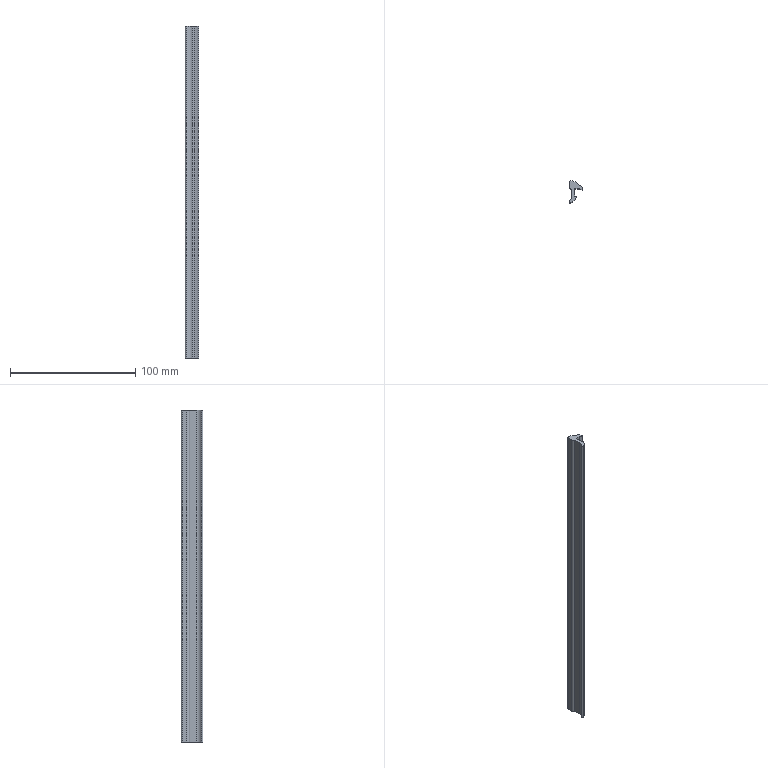Part | SolidWorks | features BaseBody 1, MoveFace 1 | 1 solid | 20 faces | box 10.8 x 17.5 x 265 mm | volume 20882 mm3 | cylinder 11 | plane 9 | commonest cylinder face diameters 1.6 x2 14 x2 0.4 x1 0.6 x1 0.8 x1 2.6 x1
STEP:
#1=CARTESIAN_POINT('',(-3.236,-11.055,165.));
#2=VERTEX_POINT('',#1);
#3=CARTESIAN_POINT('',(-4.3,-10.3,165.));
#4=VERTEX_POINT('',#3);
#5=CARTESIAN_POINT('',(-3.5,-10.3,165.));
#6=DIRECTION('',(0.,0.,-1.));
#7=DIRECTION('',(1.,0.,0.));
#8=AXIS2_PLACEMENT_3D('',#5,#6,#7);
#9=CIRCLE('',#8,0.8);
#10=EDGE_CURVE('',#2,#4,#9,.T.);
#11=ORIENTED_EDGE('',*,*,#10,.T.);
#12=CARTESIAN_POINT('',(-4.3,-10.3,-100.));
#13=VERTEX_POINT('',#12);
#14=CARTESIAN_POINT('',(-4.3,-10.3,-100.));
#15=DIRECTION('',(0.,0.,-1.));
#16=VECTOR('',#15,1000.);
#17=LINE('',#14,#16);
#18=EDGE_CURVE('',#4,#13,#17,.T.);
#19=ORIENTED_EDGE('',*,*,#18,.T.);
#20=CARTESIAN_POINT('',(-3.236,-11.055,-100.));
#21=VERTEX_POINT('',#20);
#22=CARTESIAN_POINT('',(-3.5,-10.3,-100.));
#23=DIRECTION('',(0.,0.,1.));
#24=DIRECTION('',(-1.,0.,0.));
#25=AXIS2_PLACEMENT_3D('',#22,#23,#24);
#26=CIRCLE('',#25,0.8);
#27=EDGE_CURVE('',#13,#21,#26,.T.);
#28=ORIENTED_EDGE('',*,*,#27,.T.);
#29=CARTESIAN_POINT('',(-3.236,-11.055,-100.));
#30=DIRECTION('',(0.,0.,-1.));
#31=VECTOR('',#30,1000.);
#32=LINE('',#29,#31);
#33=EDGE_CURVE('',#2,#21,#32,.T.);
#34=ORIENTED_EDGE('',*,*,#33,.F.);
#35=EDGE_LOOP('',(#11,#19,#28,#34));
#36=FACE_OUTER_BOUND('',#35,.T.);
#37=CARTESIAN_POINT('',(-3.5,-10.3,-100.));
#38=DIRECTION('',(0.,0.,-1.));
#39=DIRECTION('',(-1.,0.,0.));
#40=AXIS2_PLACEMENT_3D('',#37,#38,#39);
#41=CYLINDRICAL_SURFACE('',#40,0.8);
#42=ADVANCED_FACE('',(#36),#41,.T.);
#43=CARTESIAN_POINT('',(1.184,-6.397,-100.));
#44=VERTEX_POINT('',#43);
#45=CARTESIAN_POINT('',(-5.702,-4.29,-100.));
#46=DIRECTION('',(0.,0.,1.));
#47=DIRECTION('',(-1.,0.,0.));
#48=AXIS2_PLACEMENT_3D('',#45,#46,#47);
#49=CIRCLE('',#48,7.201);
#50=EDGE_CURVE('',#21,#44,#49,.T.);
#51=ORIENTED_EDGE('',*,*,#50,.T.);
#52=CARTESIAN_POINT('',(1.184,-6.397,165.));
#53=VERTEX_POINT('',#52);
#54=CARTESIAN_POINT('',(1.184,-6.397,-100.));
#55=DIRECTION('',(0.,0.,1.));
#56=VECTOR('',#55,1000.);
#57=LINE('',#54,#56);
#58=EDGE_CURVE('',#44,#53,#57,.T.);
#59=ORIENTED_EDGE('',*,*,#58,.T.);
#60=CARTESIAN_POINT('',(-5.702,-4.29,165.));
#61=DIRECTION('',(0.,0.,-1.));
#62=DIRECTION('',(1.,0.,0.));
#63=AXIS2_PLACEMENT_3D('',#60,#61,#62);
#64=CIRCLE('',#63,7.201);
#65=EDGE_CURVE('',#53,#2,#64,.T.);
#66=ORIENTED_EDGE('',*,*,#65,.T.);
#67=ORIENTED_EDGE('',*,*,#33,.T.);
#68=EDGE_LOOP('',(#51,#59,#66,#67));
#69=FACE_OUTER_BOUND('',#68,.T.);
#70=CARTESIAN_POINT('',(-5.702,-4.29,-100.));
#71=DIRECTION('',(0.,0.,-1.));
#72=DIRECTION('',(-1.,0.,0.));
#73=AXIS2_PLACEMENT_3D('',#70,#71,#72);
#74=CYLINDRICAL_SURFACE('',#73,7.201);
#75=ADVANCED_FACE('',(#69),#74,.T.);
#76=CARTESIAN_POINT('',(0.9,-6.,-100.));
#77=VERTEX_POINT('',#76);
#78=CARTESIAN_POINT('',(0.9,-6.3,-100.));
#79=DIRECTION('',(0.,0.,1.));
#80=DIRECTION('',(-1.,0.,0.));
#81=AXIS2_PLACEMENT_3D('',#78,#79,#80);
#82=CIRCLE('',#81,0.3);
#83=EDGE_CURVE('',#44,#77,#82,.T.);
#84=ORIENTED_EDGE('',*,*,#83,.T.);
#85=CARTESIAN_POINT('',(0.9,-6.,165.));
#86=VERTEX_POINT('',#85);
#87=CARTESIAN_POINT('',(0.9,-6.,-100.));
#88=DIRECTION('',(0.,0.,1.));
#89=VECTOR('',#88,1000.);
#90=LINE('',#87,#89);
#91=EDGE_CURVE('',#77,#86,#90,.T.);
#92=ORIENTED_EDGE('',*,*,#91,.T.);
#93=CARTESIAN_POINT('',(0.9,-6.3,165.));
#94=DIRECTION('',(0.,0.,-1.));
#95=DIRECTION('',(1.,0.,0.));
#96=AXIS2_PLACEMENT_3D('',#93,#94,#95);
#97=CIRCLE('',#96,0.3);
#98=EDGE_CURVE('',#86,#53,#97,.T.);
#99=ORIENTED_EDGE('',*,*,#98,.T.);
#100=ORIENTED_EDGE('',*,*,#58,.F.);
#101=EDGE_LOOP('',(#84,#92,#99,#100));
#102=FACE_OUTER_BOUND('',#101,.T.);
#103=CARTESIAN_POINT('',(0.9,-6.3,-100.));
#104=DIRECTION('',(0.,0.,-1.));
#105=DIRECTION('',(-1.,0.,0.));
#106=AXIS2_PLACEMENT_3D('',#103,#104,#105);
#107=CYLINDRICAL_SURFACE('',#106,0.3);
#108=ADVANCED_FACE('',(#102),#107,.T.);
#109=CARTESIAN_POINT('',(-2.5,-0.5,-100.));
#110=VERTEX_POINT('',#109);
#111=CARTESIAN_POINT('',(-2.5,-6.153,-100.));
#112=VERTEX_POINT('',#111);
#113=CARTESIAN_POINT('',(-2.5,-6.397,-100.));
#114=DIRECTION('',(0.,-1.,0.));
#115=VECTOR('',#114,1000.);
#116=LINE('',#113,#115);
#117=EDGE_CURVE('',#110,#112,#116,.T.);
#118=ORIENTED_EDGE('',*,*,#117,.F.);
#119=CARTESIAN_POINT('',(-4.2,1.695,-100.));
#120=VERTEX_POINT('',#119);
#121=CARTESIAN_POINT('',(-1.701,1.875,-100.));
#122=DIRECTION('',(0.,0.,1.));
#123=DIRECTION('',(-1.,0.,0.));
#124=AXIS2_PLACEMENT_3D('',#121,#122,#123);
#125=CIRCLE('',#124,2.506);
#126=EDGE_CURVE('',#120,#110,#125,.T.);
#127=ORIENTED_EDGE('',*,*,#126,.F.);
#128=CARTESIAN_POINT('',(-4.2,5.1,-100.));
#129=VERTEX_POINT('',#128);
#130=CARTESIAN_POINT('',(-4.2,-6.397,-100.));
#131=DIRECTION('',(0.,-1.,0.));
#132=VECTOR('',#131,1000.);
#133=LINE('',#130,#132);
#134=EDGE_CURVE('',#129,#120,#133,.T.);
#135=ORIENTED_EDGE('',*,*,#134,.F.);
#136=CARTESIAN_POINT('',(-2.892,6.4,-100.));
#137=VERTEX_POINT('',#136);
#138=CARTESIAN_POINT('',(-2.9,5.1,-100.));
#139=DIRECTION('',(0.,0.,1.));
#140=DIRECTION('',(-1.,0.,0.));
#141=AXIS2_PLACEMENT_3D('',#138,#139,#140);
#142=CIRCLE('',#141,1.3);
#143=EDGE_CURVE('',#137,#129,#142,.T.);
#144=ORIENTED_EDGE('',*,*,#143,.F.);
#145=CARTESIAN_POINT('',(0.5,5.5,-100.));
#146=VERTEX_POINT('',#145);
#147=CARTESIAN_POINT('',(-2.934,-0.5999,-100.));
#148=DIRECTION('',(0.,0.,1.));
#149=DIRECTION('',(-1.,0.,0.));
#150=AXIS2_PLACEMENT_3D('',#147,#148,#149);
#151=CIRCLE('',#150,7.);
#152=EDGE_CURVE('',#146,#137,#151,.T.);
#153=ORIENTED_EDGE('',*,*,#152,.F.);
#154=CARTESIAN_POINT('',(5.5,1.7,-100.));
#155=VERTEX_POINT('',#154);
#156=CARTESIAN_POINT('',(5.5,1.7,-100.));
#157=DIRECTION('',(-0.7962,0.6051,0.));
#158=VECTOR('',#157,1000.);
#159=LINE('',#156,#158);
#160=EDGE_CURVE('',#155,#146,#159,.T.);
#161=ORIENTED_EDGE('',*,*,#160,.F.);
#162=CARTESIAN_POINT('',(6.458,-0.2215,-100.));
#163=VERTEX_POINT('',#162);
#164=CARTESIAN_POINT('',(6.458,-0.2215,-100.));
#165=DIRECTION('',(-0.4462,0.8949,0.));
#166=VECTOR('',#165,1000.);
#167=LINE('',#164,#166);
#168=EDGE_CURVE('',#163,#155,#167,.T.);
#169=ORIENTED_EDGE('',*,*,#168,.F.);
#170=CARTESIAN_POINT('',(5.895,-0.7433,-100.));
#171=VERTEX_POINT('',#170);
#172=CARTESIAN_POINT('',(6.1,-0.4,-100.));
#173=DIRECTION('',(0.,0.,1.));
#174=DIRECTION('',(-1.,0.,0.));
#175=AXIS2_PLACEMENT_3D('',#172,#173,#174);
#176=CIRCLE('',#175,0.4);
#177=EDGE_CURVE('',#171,#163,#176,.T.);
#178=ORIENTED_EDGE('',*,*,#177,.F.);
#179=CARTESIAN_POINT('',(3.,0.,-100.));
#180=VERTEX_POINT('',#179);
#181=CARTESIAN_POINT('',(2.746,-6.995,-100.));
#182=DIRECTION('',(0.,0.,-1.));
#183=DIRECTION('',(-1.,0.,0.));
#184=AXIS2_PLACEMENT_3D('',#181,#182,#183);
#185=CIRCLE('',#184,7.);
#186=EDGE_CURVE('',#180,#171,#185,.T.);
#187=ORIENTED_EDGE('',*,*,#186,.F.);
#188=CARTESIAN_POINT('',(0.,0.,-100.));
#189=VERTEX_POINT('',#188);
#190=CARTESIAN_POINT('',(-6.814,0.,-100.));
#191=DIRECTION('',(1.,0.,0.));
#192=VECTOR('',#191,1000.);
#193=LINE('',#190,#192);
#194=EDGE_CURVE('',#189,#180,#193,.T.);
#195=ORIENTED_EDGE('',*,*,#194,.F.);
#196=CARTESIAN_POINT('',(0.,-5.8,-100.));
#197=VERTEX_POINT('',#196);
#198=CARTESIAN_POINT('',(0.,-6.397,-100.));
#199=DIRECTION('',(0.,1.,0.));
#200=VECTOR('',#199,1000.);
#201=LINE('',#198,#200);
#202=EDGE_CURVE('',#197,#189,#201,.T.);
#203=ORIENTED_EDGE('',*,*,#202,.F.);
#204=CARTESIAN_POINT('',(0.2,-6.,-100.));
#205=VERTEX_POINT('',#204);
#206=CARTESIAN_POINT('',(0.2,-5.8,-100.));
#207=DIRECTION('',(0.,0.,1.));
#208=DIRECTION('',(-1.,0.,0.));
#209=AXIS2_PLACEMENT_3D('',#206,#207,#208);
#210=CIRCLE('',#209,0.2);
#211=EDGE_CURVE('',#197,#205,#210,.T.);
#212=ORIENTED_EDGE('',*,*,#211,.T.);
#213=CARTESIAN_POINT('',(-6.814,-6.,-100.));
#214=DIRECTION('',(-1.,0.,0.));
#215=VECTOR('',#214,1000.);
#216=LINE('',#213,#215);
#217=EDGE_CURVE('',#77,#205,#216,.T.);
#218=ORIENTED_EDGE('',*,*,#217,.F.);
#219=ORIENTED_EDGE('',*,*,#83,.F.);
#220=ORIENTED_EDGE('',*,*,#50,.F.);
#221=ORIENTED_EDGE('',*,*,#27,.F.);
#222=CARTESIAN_POINT('',(-3.998,-9.674,-100.));
#223=VERTEX_POINT('',#222);
#224=CARTESIAN_POINT('',(-3.5,-10.3,-100.));
#225=DIRECTION('',(0.,0.,1.));
#226=DIRECTION('',(-1.,0.,0.));
#227=AXIS2_PLACEMENT_3D('',#224,#225,#226);
#228=CIRCLE('',#227,0.8);
#229=EDGE_CURVE('',#223,#13,#228,.T.);
#230=ORIENTED_EDGE('',*,*,#229,.F.);
#231=CARTESIAN_POINT('',(-6.814,-6.397,-100.));
#232=DIRECTION('',(0.,0.,-1.));
#233=DIRECTION('',(-1.,0.,0.));
#234=AXIS2_PLACEMENT_3D('',#231,#232,#233);
#235=CIRCLE('',#234,4.321);
#236=EDGE_CURVE('',#112,#223,#235,.T.);
#237=ORIENTED_EDGE('',*,*,#236,.F.);
#238=EDGE_LOOP('',(#118,#127,#135,#144,#153,#161,#169,#178,#187,#195,#203,#212,#218,#219,#220,#221,#230,#237));
#239=FACE_OUTER_BOUND('',#238,.T.);
#240=CARTESIAN_POINT('',(-6.814,-6.397,-100.));
#241=DIRECTION('',(0.,0.,1.));
#242=DIRECTION('',(1.,0.,0.));
#243=AXIS2_PLACEMENT_3D('',#240,#241,#242);
#244=PLANE('',#243);
#245=ADVANCED_FACE('',(#239),#244,.F.);
#246=ORIENTED_EDGE('',*,*,#18,.F.);
#247=CARTESIAN_POINT('',(-3.998,-9.674,165.));
#248=VERTEX_POINT('',#247);
#249=CARTESIAN_POINT('',(-3.5,-10.3,165.));
#250=DIRECTION('',(0.,0.,-1.));
#251=DIRECTION('',(1.,0.,0.));
#252=AXIS2_PLACEMENT_3D('',#249,#250,#251);
#253=CIRCLE('',#252,0.8);
#254=EDGE_CURVE('',#4,#248,#253,.T.);
#255=ORIENTED_EDGE('',*,*,#254,.T.);
#256=CARTESIAN_POINT('',(-3.998,-9.674,-100.));
#257=DIRECTION('',(0.,0.,-1.));
#258=VECTOR('',#257,1000.);
#259=LINE('',#256,#258);
#260=EDGE_CURVE('',#248,#223,#259,.T.);
#261=ORIENTED_EDGE('',*,*,#260,.T.);
#262=ORIENTED_EDGE('',*,*,#229,.T.);
#263=EDGE_LOOP('',(#246,#255,#261,#262));
#264=FACE_OUTER_BOUND('',#263,.T.);
#265=CARTESIAN_POINT('',(-3.5,-10.3,-100.));
#266=DIRECTION('',(0.,0.,-1.));
#267=DIRECTION('',(-1.,0.,0.));
#268=AXIS2_PLACEMENT_3D('',#265,#266,#267);
#269=CYLINDRICAL_SURFACE('',#268,0.8);
#270=ADVANCED_FACE('',(#264),#269,.T.);
#271=CARTESIAN_POINT('',(-4.2,1.695,165.));
#272=VERTEX_POINT('',#271);
#273=CARTESIAN_POINT('',(-2.5,-0.5,165.));
#274=VERTEX_POINT('',#273);
#275=CARTESIAN_POINT('',(-1.701,1.875,165.));
#276=DIRECTION('',(0.,0.,1.));
#277=DIRECTION('',(1.,0.,0.));
#278=AXIS2_PLACEMENT_3D('',#275,#276,#277);
#279=CIRCLE('',#278,2.506);
#280=EDGE_CURVE('',#272,#274,#279,.T.);
#281=ORIENTED_EDGE('',*,*,#280,.T.);
#282=CARTESIAN_POINT('',(-2.5,-6.153,165.));
#283=VERTEX_POINT('',#282);
#284=CARTESIAN_POINT('',(-2.5,-6.397,165.));
#285=DIRECTION('',(0.,-1.,0.));
#286=VECTOR('',#285,1000.);
#287=LINE('',#284,#286);
#288=EDGE_CURVE('',#274,#283,#287,.T.);
#289=ORIENTED_EDGE('',*,*,#288,.T.);
#290=CARTESIAN_POINT('',(-6.814,-6.397,165.));
#291=DIRECTION('',(0.,0.,-1.));
#292=DIRECTION('',(1.,0.,0.));
#293=AXIS2_PLACEMENT_3D('',#290,#291,#292);
#294=CIRCLE('',#293,4.321);
#295=EDGE_CURVE('',#283,#248,#294,.T.);
#296=ORIENTED_EDGE('',*,*,#295,.T.);
#297=ORIENTED_EDGE('',*,*,#254,.F.);
#298=ORIENTED_EDGE('',*,*,#10,.F.);
#299=ORIENTED_EDGE('',*,*,#65,.F.);
#300=ORIENTED_EDGE('',*,*,#98,.F.);
#301=CARTESIAN_POINT('',(0.2,-6.,165.));
#302=VERTEX_POINT('',#301);
#303=CARTESIAN_POINT('',(-6.814,-6.,165.));
#304=DIRECTION('',(-1.,0.,0.));
#305=VECTOR('',#304,1000.);
#306=LINE('',#303,#305);
#307=EDGE_CURVE('',#86,#302,#306,.T.);
#308=ORIENTED_EDGE('',*,*,#307,.T.);
#309=CARTESIAN_POINT('',(0.,-5.8,165.));
#310=VERTEX_POINT('',#309);
#311=CARTESIAN_POINT('',(0.2,-5.8,165.));
#312=DIRECTION('',(0.,0.,-1.));
#313=DIRECTION('',(1.,0.,0.));
#314=AXIS2_PLACEMENT_3D('',#311,#312,#313);
#315=CIRCLE('',#314,0.2);
#316=EDGE_CURVE('',#302,#310,#315,.T.);
#317=ORIENTED_EDGE('',*,*,#316,.T.);
#318=CARTESIAN_POINT('',(0.,0.,165.));
#319=VERTEX_POINT('',#318);
#320=CARTESIAN_POINT('',(0.,-6.397,165.));
#321=DIRECTION('',(0.,1.,0.));
#322=VECTOR('',#321,1000.);
#323=LINE('',#320,#322);
#324=EDGE_CURVE('',#310,#319,#323,.T.);
#325=ORIENTED_EDGE('',*,*,#324,.T.);
#326=CARTESIAN_POINT('',(3.,0.,165.));
#327=VERTEX_POINT('',#326);
#328=CARTESIAN_POINT('',(-6.814,0.,165.));
#329=DIRECTION('',(1.,0.,0.));
#330=VECTOR('',#329,1000.);
#331=LINE('',#328,#330);
#332=EDGE_CURVE('',#319,#327,#331,.T.);
#333=ORIENTED_EDGE('',*,*,#332,.T.);
#334=CARTESIAN_POINT('',(5.895,-0.7433,165.));
#335=VERTEX_POINT('',#334);
#336=CARTESIAN_POINT('',(2.746,-6.995,165.));
#337=DIRECTION('',(0.,0.,-1.));
#338=DIRECTION('',(1.,0.,0.));
#339=AXIS2_PLACEMENT_3D('',#336,#337,#338);
#340=CIRCLE('',#339,7.);
#341=EDGE_CURVE('',#327,#335,#340,.T.);
#342=ORIENTED_EDGE('',*,*,#341,.T.);
#343=CARTESIAN_POINT('',(6.458,-0.2215,165.));
#344=VERTEX_POINT('',#343);
#345=CARTESIAN_POINT('',(6.1,-0.4,165.));
#346=DIRECTION('',(0.,0.,-1.));
#347=DIRECTION('',(1.,0.,0.));
#348=AXIS2_PLACEMENT_3D('',#345,#346,#347);
#349=CIRCLE('',#348,0.4);
#350=EDGE_CURVE('',#344,#335,#349,.T.);
#351=ORIENTED_EDGE('',*,*,#350,.F.);
#352=CARTESIAN_POINT('',(5.5,1.7,165.));
#353=VERTEX_POINT('',#352);
#354=CARTESIAN_POINT('',(6.282,0.1323,165.));
#355=DIRECTION('',(-0.4462,0.8949,0.));
#356=VECTOR('',#355,1000.);
#357=LINE('',#354,#356);
#358=EDGE_CURVE('',#344,#353,#357,.T.);
#359=ORIENTED_EDGE('',*,*,#358,.T.);
#360=CARTESIAN_POINT('',(0.5,5.5,165.));
#361=VERTEX_POINT('',#360);
#362=CARTESIAN_POINT('',(1.595,4.668,165.));
#363=DIRECTION('',(-0.7962,0.6051,0.));
#364=VECTOR('',#363,1000.);
#365=LINE('',#362,#364);
#366=EDGE_CURVE('',#353,#361,#365,.T.);
#367=ORIENTED_EDGE('',*,*,#366,.T.);
#368=CARTESIAN_POINT('',(-2.892,6.4,165.));
#369=VERTEX_POINT('',#368);
#370=CARTESIAN_POINT('',(-2.934,-0.5999,165.));
#371=DIRECTION('',(0.,0.,1.));
#372=DIRECTION('',(1.,0.,0.));
#373=AXIS2_PLACEMENT_3D('',#370,#371,#372);
#374=CIRCLE('',#373,7.);
#375=EDGE_CURVE('',#361,#369,#374,.T.);
#376=ORIENTED_EDGE('',*,*,#375,.T.);
#377=CARTESIAN_POINT('',(-4.2,5.1,165.));
#378=VERTEX_POINT('',#377);
#379=CARTESIAN_POINT('',(-2.9,5.1,165.));
#380=DIRECTION('',(0.,0.,1.));
#381=DIRECTION('',(1.,0.,0.));
#382=AXIS2_PLACEMENT_3D('',#379,#380,#381);
#383=CIRCLE('',#382,1.3);
#384=EDGE_CURVE('',#369,#378,#383,.T.);
#385=ORIENTED_EDGE('',*,*,#384,.T.);
#386=CARTESIAN_POINT('',(-4.2,-6.397,165.));
#387=DIRECTION('',(0.,-1.,0.));
#388=VECTOR('',#387,1000.);
#389=LINE('',#386,#388);
#390=EDGE_CURVE('',#378,#272,#389,.T.);
#391=ORIENTED_EDGE('',*,*,#390,.T.);
#392=EDGE_LOOP('',(#281,#289,#296,#297,#298,#299,#300,#308,#317,#325,#333,#342,#351,#359,#367,#376,#385,#391));
#393=FACE_OUTER_BOUND('',#392,.T.);
#394=CARTESIAN_POINT('',(-6.814,-6.397,165.));
#395=DIRECTION('',(0.,0.,1.));
#396=DIRECTION('',(1.,0.,0.));
#397=AXIS2_PLACEMENT_3D('',#394,#395,#396);
#398=PLANE('',#397);
#399=ADVANCED_FACE('',(#393),#398,.T.);
#400=ORIENTED_EDGE('',*,*,#217,.T.);
#401=CARTESIAN_POINT('',(0.2,-6.,-100.));
#402=DIRECTION('',(0.,0.,1.));
#403=VECTOR('',#402,1000.);
#404=LINE('',#401,#403);
#405=EDGE_CURVE('',#205,#302,#404,.T.);
#406=ORIENTED_EDGE('',*,*,#405,.T.);
#407=ORIENTED_EDGE('',*,*,#307,.F.);
#408=ORIENTED_EDGE('',*,*,#91,.F.);
#409=EDGE_LOOP('',(#400,#406,#407,#408));
#410=FACE_OUTER_BOUND('',#409,.T.);
#411=CARTESIAN_POINT('',(0.9,-6.,-100.));
#412=DIRECTION('',(0.,1.,0.));
#413=DIRECTION('',(0.,0.,1.));
#414=AXIS2_PLACEMENT_3D('',#411,#412,#413);
#415=PLANE('',#414);
#416=ADVANCED_FACE('',(#410),#415,.T.);
#417=CARTESIAN_POINT('',(-2.5,-6.153,-100.));
#418=DIRECTION('',(0.,0.,1.));
#419=VECTOR('',#418,1000.);
#420=LINE('',#417,#419);
#421=EDGE_CURVE('',#112,#283,#420,.T.);
#422=ORIENTED_EDGE('',*,*,#421,.F.);
#423=ORIENTED_EDGE('',*,*,#236,.T.);
#424=ORIENTED_EDGE('',*,*,#260,.F.);
#425=ORIENTED_EDGE('',*,*,#295,.F.);
#426=EDGE_LOOP('',(#422,#423,#424,#425));
#427=FACE_OUTER_BOUND('',#426,.T.);
#428=CARTESIAN_POINT('',(-6.814,-6.397,-100.));
#429=DIRECTION('',(0.,0.,-1.));
#430=DIRECTION('',(-1.,0.,0.));
#431=AXIS2_PLACEMENT_3D('',#428,#429,#430);
#432=CYLINDRICAL_SURFACE('',#431,4.321);
#433=ADVANCED_FACE('',(#427),#432,.F.);
#434=ORIENTED_EDGE('',*,*,#117,.T.);
#435=ORIENTED_EDGE('',*,*,#421,.T.);
#436=ORIENTED_EDGE('',*,*,#288,.F.);
#437=CARTESIAN_POINT('',(-2.5,-0.5,-100.));
#438=DIRECTION('',(0.,0.,-1.));
#439=VECTOR('',#438,1000.);
#440=LINE('',#437,#439);
#441=EDGE_CURVE('',#274,#110,#440,.T.);
#442=ORIENTED_EDGE('',*,*,#441,.T.);
#443=EDGE_LOOP('',(#434,#435,#436,#442));
#444=FACE_OUTER_BOUND('',#443,.T.);
#445=CARTESIAN_POINT('',(-2.5,-0.5,-100.));
#446=DIRECTION('',(-1.,0.,0.));
#447=DIRECTION('',(0.,0.,1.));
#448=AXIS2_PLACEMENT_3D('',#445,#446,#447);
#449=PLANE('',#448);
#450=ADVANCED_FACE('',(#444),#449,.T.);
#451=ORIENTED_EDGE('',*,*,#126,.T.);
#452=ORIENTED_EDGE('',*,*,#441,.F.);
#453=ORIENTED_EDGE('',*,*,#280,.F.);
#454=CARTESIAN_POINT('',(-4.2,1.695,-100.));
#455=DIRECTION('',(0.,0.,-1.));
#456=VECTOR('',#455,1000.);
#457=LINE('',#454,#456);
#458=EDGE_CURVE('',#272,#120,#457,.T.);
#459=ORIENTED_EDGE('',*,*,#458,.T.);
#460=EDGE_LOOP('',(#451,#452,#453,#459));
#461=FACE_OUTER_BOUND('',#460,.T.);
#462=CARTESIAN_POINT('',(-1.701,1.875,-100.));
#463=DIRECTION('',(0.,0.,-1.));
#464=DIRECTION('',(-1.,0.,0.));
#465=AXIS2_PLACEMENT_3D('',#462,#463,#464);
#466=CYLINDRICAL_SURFACE('',#465,2.506);
#467=ADVANCED_FACE('',(#461),#466,.T.);
#468=ORIENTED_EDGE('',*,*,#134,.T.);
#469=ORIENTED_EDGE('',*,*,#458,.F.);
#470=ORIENTED_EDGE('',*,*,#390,.F.);
#471=CARTESIAN_POINT('',(-4.2,5.1,-100.));
#472=DIRECTION('',(0.,0.,-1.));
#473=VECTOR('',#472,1000.);
#474=LINE('',#471,#473);
#475=EDGE_CURVE('',#378,#129,#474,.T.);
#476=ORIENTED_EDGE('',*,*,#475,.T.);
#477=EDGE_LOOP('',(#468,#469,#470,#476));
#478=FACE_OUTER_BOUND('',#477,.T.);
#479=CARTESIAN_POINT('',(-4.2,5.1,-100.));
#480=DIRECTION('',(-1.,0.,0.));
#481=DIRECTION('',(0.,0.,1.));
#482=AXIS2_PLACEMENT_3D('',#479,#480,#481);
#483=PLANE('',#482);
#484=ADVANCED_FACE('',(#478),#483,.T.);
#485=ORIENTED_EDGE('',*,*,#143,.T.);
#486=ORIENTED_EDGE('',*,*,#475,.F.);
#487=ORIENTED_EDGE('',*,*,#384,.F.);
#488=CARTESIAN_POINT('',(-2.892,6.4,-100.));
#489=DIRECTION('',(0.,0.,-1.));
#490=VECTOR('',#489,1000.);
#491=LINE('',#488,#490);
#492=EDGE_CURVE('',#369,#137,#491,.T.);
#493=ORIENTED_EDGE('',*,*,#492,.T.);
#494=EDGE_LOOP('',(#485,#486,#487,#493));
#495=FACE_OUTER_BOUND('',#494,.T.);
#496=CARTESIAN_POINT('',(-2.9,5.1,-100.));
#497=DIRECTION('',(0.,0.,-1.));
#498=DIRECTION('',(-1.,0.,0.));
#499=AXIS2_PLACEMENT_3D('',#496,#497,#498);
#500=CYLINDRICAL_SURFACE('',#499,1.3);
#501=ADVANCED_FACE('',(#495),#500,.T.);
#502=ORIENTED_EDGE('',*,*,#152,.T.);
#503=ORIENTED_EDGE('',*,*,#492,.F.);
#504=ORIENTED_EDGE('',*,*,#375,.F.);
#505=CARTESIAN_POINT('',(0.5,5.5,-100.));
#506=DIRECTION('',(0.,0.,-1.));
#507=VECTOR('',#506,1000.);
#508=LINE('',#505,#507);
#509=EDGE_CURVE('',#361,#146,#508,.T.);
#510=ORIENTED_EDGE('',*,*,#509,.T.);
#511=EDGE_LOOP('',(#502,#503,#504,#510));
#512=FACE_OUTER_BOUND('',#511,.T.);
#513=CARTESIAN_POINT('',(-2.934,-0.5999,-100.));
#514=DIRECTION('',(0.,0.,-1.));
#515=DIRECTION('',(-1.,0.,0.));
#516=AXIS2_PLACEMENT_3D('',#513,#514,#515);
#517=CYLINDRICAL_SURFACE('',#516,7.);
#518=ADVANCED_FACE('',(#512),#517,.T.);
#519=ORIENTED_EDGE('',*,*,#160,.T.);
#520=ORIENTED_EDGE('',*,*,#509,.F.);
#521=ORIENTED_EDGE('',*,*,#366,.F.);
#522=CARTESIAN_POINT('',(5.5,1.7,-100.));
#523=DIRECTION('',(0.,0.,-1.));
#524=VECTOR('',#523,1000.);
#525=LINE('',#522,#524);
#526=EDGE_CURVE('',#353,#155,#525,.T.);
#527=ORIENTED_EDGE('',*,*,#526,.T.);
#528=EDGE_LOOP('',(#519,#520,#521,#527));
#529=FACE_OUTER_BOUND('',#528,.T.);
#530=CARTESIAN_POINT('',(5.5,1.7,-100.));
#531=DIRECTION('',(0.6051,0.7962,0.));
#532=DIRECTION('',(-0.7962,0.6051,0.));
#533=AXIS2_PLACEMENT_3D('',#530,#531,#532);
#534=PLANE('',#533);
#535=ADVANCED_FACE('',(#529),#534,.T.);
#536=ORIENTED_EDGE('',*,*,#168,.T.);
#537=ORIENTED_EDGE('',*,*,#526,.F.);
#538=ORIENTED_EDGE('',*,*,#358,.F.);
#539=CARTESIAN_POINT('',(6.458,-0.2215,-100.));
#540=DIRECTION('',(0.,0.,-1.));
#541=VECTOR('',#540,1000.);
#542=LINE('',#539,#541);
#543=EDGE_CURVE('',#344,#163,#542,.T.);
#544=ORIENTED_EDGE('',*,*,#543,.T.);
#545=EDGE_LOOP('',(#536,#537,#538,#544));
#546=FACE_OUTER_BOUND('',#545,.T.);
#547=CARTESIAN_POINT('',(6.458,-0.2215,-100.));
#548=DIRECTION('',(0.8949,0.4462,0.));
#549=DIRECTION('',(-0.4462,0.8949,0.));
#550=AXIS2_PLACEMENT_3D('',#547,#548,#549);
#551=PLANE('',#550);
#552=ADVANCED_FACE('',(#546),#551,.T.);
#553=CARTESIAN_POINT('',(3.,0.,-100.));
#554=DIRECTION('',(0.,0.,1.));
#555=VECTOR('',#554,1000.);
#556=LINE('',#553,#555);
#557=EDGE_CURVE('',#180,#327,#556,.T.);
#558=ORIENTED_EDGE('',*,*,#557,.F.);
#559=ORIENTED_EDGE('',*,*,#186,.T.);
#560=CARTESIAN_POINT('',(5.895,-0.7433,-100.));
#561=DIRECTION('',(0.,0.,-1.));
#562=VECTOR('',#561,1000.);
#563=LINE('',#560,#562);
#564=EDGE_CURVE('',#335,#171,#563,.T.);
#565=ORIENTED_EDGE('',*,*,#564,.F.);
#566=ORIENTED_EDGE('',*,*,#341,.F.);
#567=EDGE_LOOP('',(#558,#559,#565,#566));
#568=FACE_OUTER_BOUND('',#567,.T.);
#569=CARTESIAN_POINT('',(2.746,-6.995,-100.));
#570=DIRECTION('',(0.,0.,-1.));
#571=DIRECTION('',(-1.,0.,0.));
#572=AXIS2_PLACEMENT_3D('',#569,#570,#571);
#573=CYLINDRICAL_SURFACE('',#572,7.);
#574=ADVANCED_FACE('',(#568),#573,.F.);
#575=ORIENTED_EDGE('',*,*,#194,.T.);
#576=ORIENTED_EDGE('',*,*,#557,.T.);
#577=ORIENTED_EDGE('',*,*,#332,.F.);
#578=CARTESIAN_POINT('',(0.,0.,-100.));
#579=DIRECTION('',(0.,0.,-1.));
#580=VECTOR('',#579,1000.);
#581=LINE('',#578,#580);
#582=EDGE_CURVE('',#319,#189,#581,.T.);
#583=ORIENTED_EDGE('',*,*,#582,.T.);
#584=EDGE_LOOP('',(#575,#576,#577,#583));
#585=FACE_OUTER_BOUND('',#584,.T.);
#586=CARTESIAN_POINT('',(0.,0.,-100.));
#587=DIRECTION('',(0.,-1.,0.));
#588=DIRECTION('',(0.,0.,-1.));
#589=AXIS2_PLACEMENT_3D('',#586,#587,#588);
#590=PLANE('',#589);
#591=ADVANCED_FACE('',(#585),#590,.T.);
#592=ORIENTED_EDGE('',*,*,#202,.T.);
#593=ORIENTED_EDGE('',*,*,#582,.F.);
#594=ORIENTED_EDGE('',*,*,#324,.F.);
#595=CARTESIAN_POINT('',(0.,-5.8,-100.));
#596=DIRECTION('',(0.,0.,-1.));
#597=VECTOR('',#596,1000.);
#598=LINE('',#595,#597);
#599=EDGE_CURVE('',#310,#197,#598,.T.);
#600=ORIENTED_EDGE('',*,*,#599,.T.);
#601=EDGE_LOOP('',(#592,#593,#594,#600));
#602=FACE_OUTER_BOUND('',#601,.T.);
#603=CARTESIAN_POINT('',(0.,-5.8,-100.));
#604=DIRECTION('',(1.,0.,0.));
#605=DIRECTION('',(0.,0.,-1.));
#606=AXIS2_PLACEMENT_3D('',#603,#604,#605);
#607=PLANE('',#606);
#608=ADVANCED_FACE('',(#602),#607,.T.);
#609=ORIENTED_EDGE('',*,*,#405,.F.);
#610=ORIENTED_EDGE('',*,*,#211,.F.);
#611=ORIENTED_EDGE('',*,*,#599,.F.);
#612=ORIENTED_EDGE('',*,*,#316,.F.);
#613=EDGE_LOOP('',(#609,#610,#611,#612));
#614=FACE_OUTER_BOUND('',#613,.T.);
#615=CARTESIAN_POINT('',(0.2,-5.8,-100.));
#616=DIRECTION('',(0.,0.,-1.));
#617=DIRECTION('',(-1.,0.,0.));
#618=AXIS2_PLACEMENT_3D('',#615,#616,#617);
#619=CYLINDRICAL_SURFACE('',#618,0.2);
#620=ADVANCED_FACE('',(#614),#619,.F.);
#621=ORIENTED_EDGE('',*,*,#177,.T.);
#622=ORIENTED_EDGE('',*,*,#543,.F.);
#623=ORIENTED_EDGE('',*,*,#350,.T.);
#624=ORIENTED_EDGE('',*,*,#564,.T.);
#625=EDGE_LOOP('',(#621,#622,#623,#624));
#626=FACE_OUTER_BOUND('',#625,.T.);
#627=CARTESIAN_POINT('',(6.1,-0.4,-100.));
#628=DIRECTION('',(0.,0.,-1.));
#629=DIRECTION('',(-1.,0.,0.));
#630=AXIS2_PLACEMENT_3D('',#627,#628,#629);
#631=CYLINDRICAL_SURFACE('',#630,0.4);
#632=ADVANCED_FACE('',(#626),#631,.T.);
#633=CLOSED_SHELL('',(#42,#75,#108,#245,#270,#399,#416,#433,#450,#467,#484,#501,#518,#535,#552,#574,#591,#608,#620,#632));
#634=MANIFOLD_SOLID_BREP('',#633);
#635=CARTESIAN_POINT('',(0.,0.,0.));
#636=DIRECTION('',(0.,0.,1.));
#637=DIRECTION('',(1.,0.,0.));
#638=AXIS2_PLACEMENT_3D('',#635,#636,#637);
#639=(LENGTH_UNIT()NAMED_UNIT(*)SI_UNIT(.MILLI.,.METRE.));
#640=UNCERTAINTY_MEASURE_WITH_UNIT(LENGTH_MEASURE(0.00001),#639,'','');
#641=(NAMED_UNIT(*)PLANE_ANGLE_UNIT()SI_UNIT($,.RADIAN.));
#642=(NAMED_UNIT(*)SI_UNIT($,.STERADIAN.)SOLID_ANGLE_UNIT());
#643=(GEOMETRIC_REPRESENTATION_CONTEXT(3)GLOBAL_UNCERTAINTY_ASSIGNED_CONTEXT((#640))GLOBAL_UNIT_ASSIGNED_CONTEXT((#639,#641,#642))REPRESENTATION_CONTEXT('',''));
#644=ADVANCED_BREP_SHAPE_REPRESENTATION('',(#634,#638),#643);